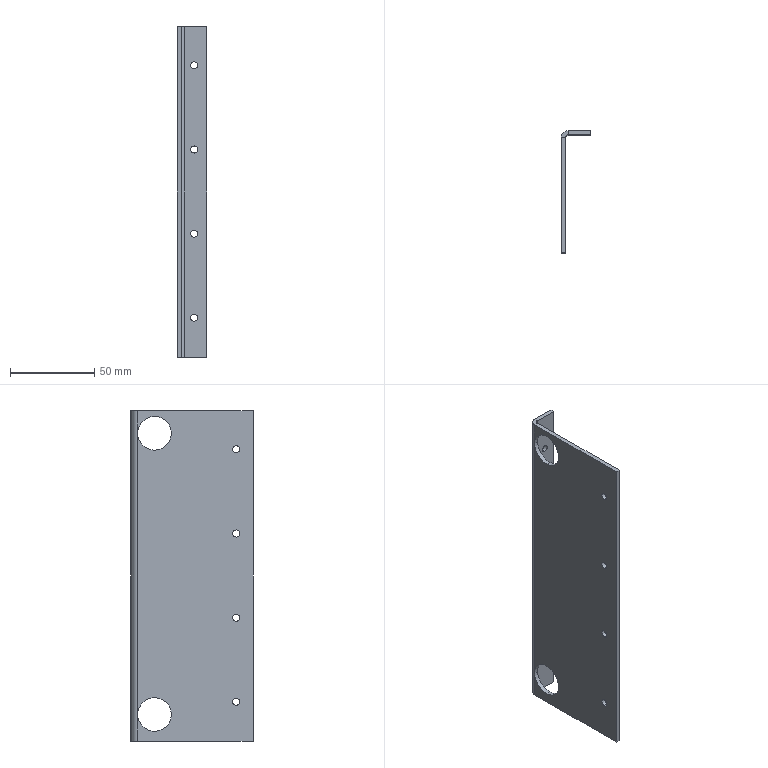Part | STEP file | 64605500 | 1 solid | 36 faces | box 17.5 x 72.5 x 196.5 mm | volume 40557 mm3 | cylinder 24 | plane 12 | commonest cylinder face diameters 4.2 x16 20 x6 3 x1 8 x1